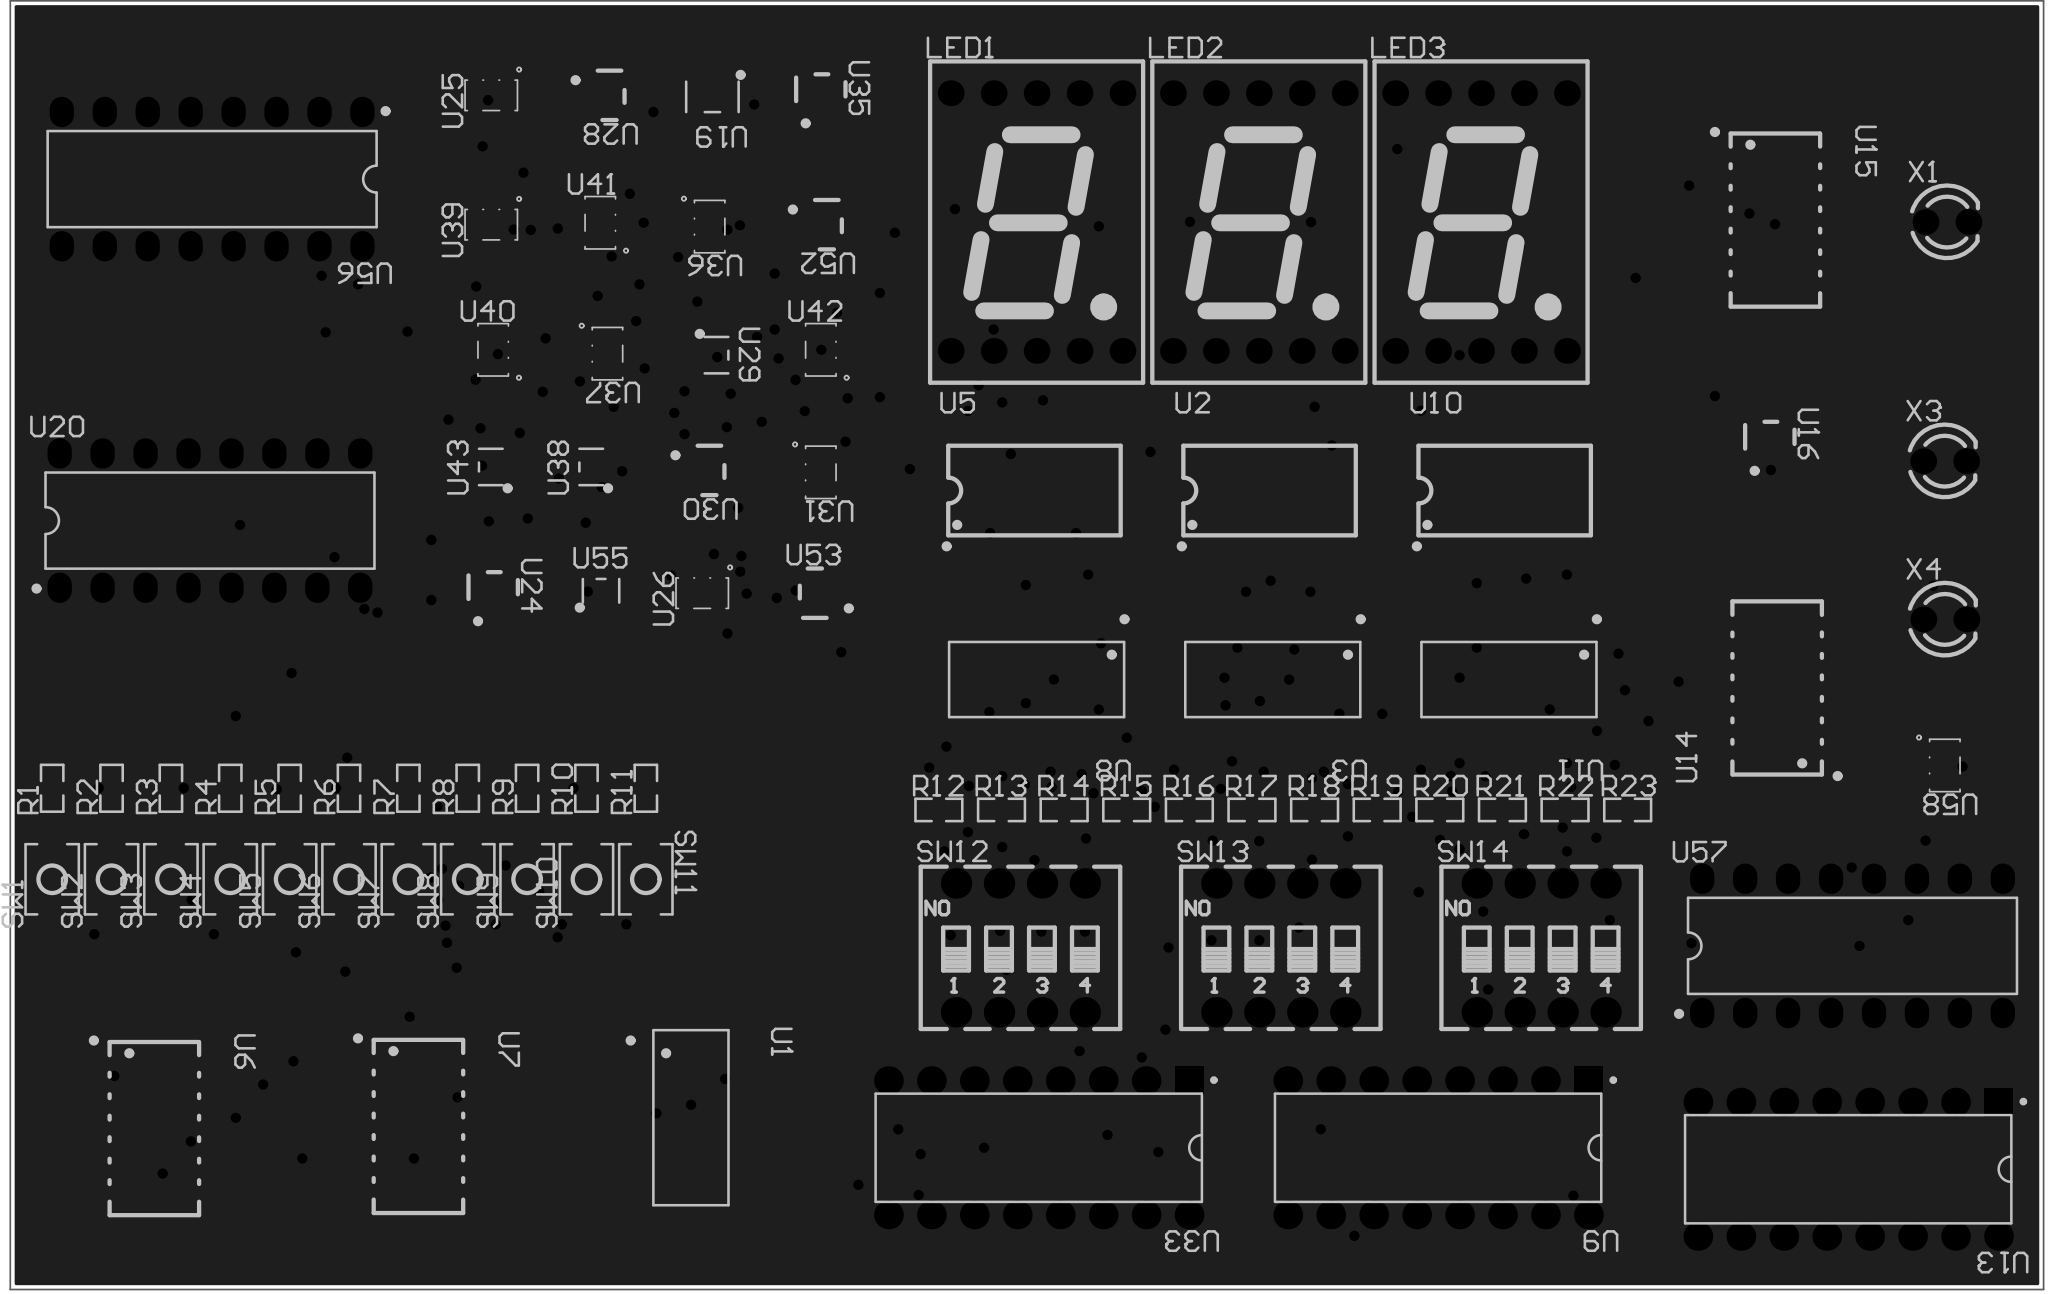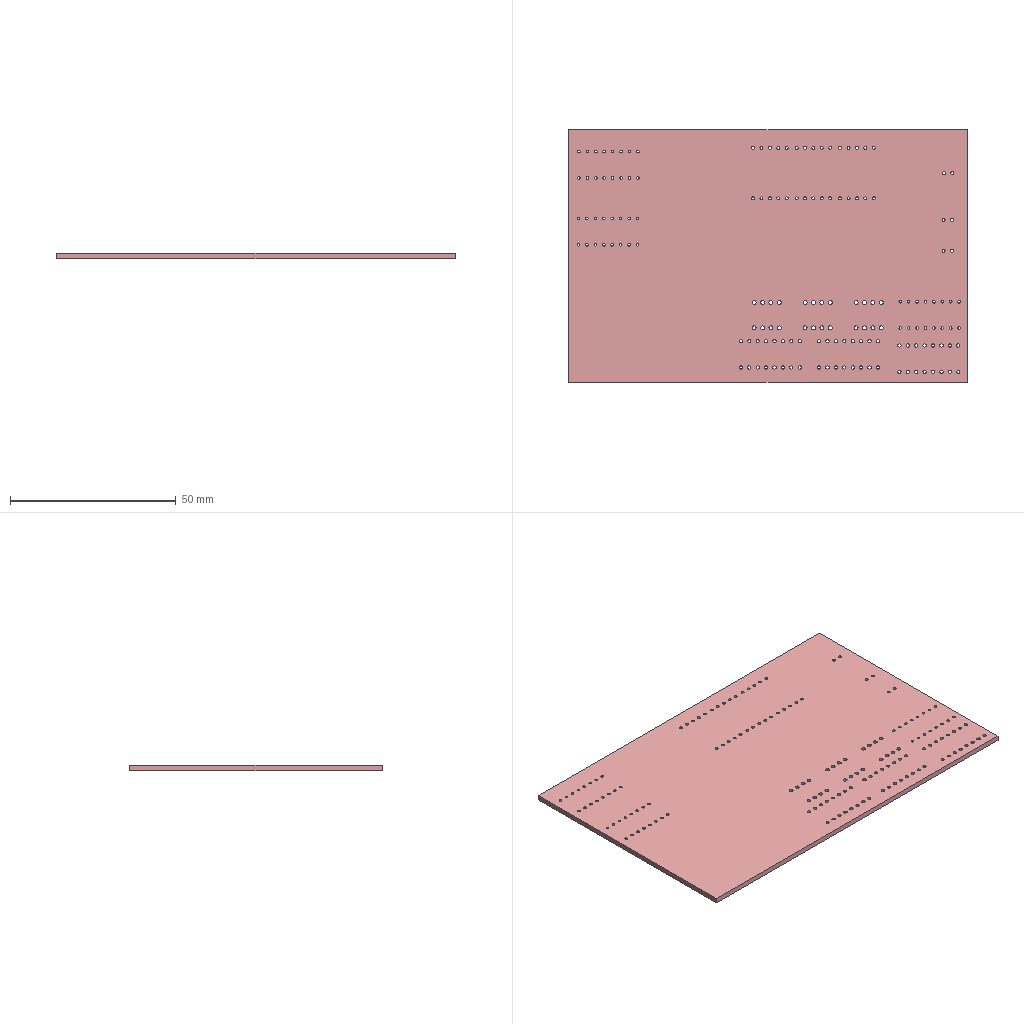Circuit board layout | Altium Designer | box 120.3 x 76.2 x 1.6 mm
Layer stack:
# Altium Designer layer stack of  (unit mm; dielectric type: 0 none, 1 core, 2 prepreg, 3 surface material)
index,name,kind,layer,copper_thickness_mm,dielectric_type,dielectric_thickness_mm,dielectric_material,dielectric_constant
0,Top Paste Mask Layer,other,,,,,,
1,Top Silkscreen Layer,other,,,,,,
2,Top Solder Mask Layer,dielectric,,,3,0.01,,3.3
3,Top Layer,copper,Top Layer,0.035,,,,
4,Dielectric1,dielectric,,,3,1.51,FR4,4.5
5,Bottom Layer,copper,Bottom Layer,0.035,,,,
6,Bottom Solder Mask Layer,dielectric,,,3,0.01,,3.3
7,Bottom Silkscreen Layer,other,,,,,,
8,Bottom Paste Mask Layer,other,,,,,,
# drill layer pairs: low layer,high layer
drill_pair,Top Layer,Bottom Layer
Part placement:
Designator,Comment,Layer,Footprint,Center-X(mm),Center-Y(mm),Rotation
LED1,,TopLayer,LED-SEG-TH_10P-L12.6-W19.0-P2.54-S15.24-BL,140.716,142.24,0
LED2,,TopLayer,LED-SEG-TH_10P-L12.6-W19.0-P2.54-S15.24-BL,153.861,142.24,0
LED3,,TopLayer,LED-SEG-TH_10P-L12.6-W19.0-P2.54-S15.24-BL,167.005,142.24,0
R1,1K,TopLayer,R0603,82.487,108.76,90
R2,1K,TopLayer,R0603,85.999,108.76,90
R3,1K,TopLayer,R0603,89.51,108.76,90
R4,1K,TopLayer,R0603,93.022,108.76,90
R5,1K,TopLayer,R0603,96.533,108.76,90
R6,1K,TopLayer,R0603,100.045,108.76,90
R7,1K,TopLayer,R0603,103.556,108.76,90
R8,1K,TopLayer,R0603,107.068,108.76,90
R9,1K,TopLayer,R0603,110.579,108.76,90
R10,1K,TopLayer,R0603,114.091,108.76,90
R11,1K,TopLayer,R0603,117.602,108.76,90
R12,1K,TopLayer,R0603,134.936,107.478,0
R13,1K,TopLayer,R0603,138.639,107.478,0
R14,1K,TopLayer,R0603,142.343,107.478,0
R15,1K,TopLayer,R0603,146.047,107.478,0
R16,1K,TopLayer,R0603,149.751,107.478,0
R17,1K,TopLayer,R0603,153.455,107.478,0
R18,1K,TopLayer,R0603,157.158,107.478,0
R19,1K,TopLayer,R0603,160.862,107.478,0
R20,1K,TopLayer,R0603,164.566,107.478,0
R21,1K,TopLayer,R0603,168.27,107.478,0
R22,1K,TopLayer,R0603,171.974,107.478,0
R23,1K,TopLayer,R0603,175.677,107.478,0
SW1,轻触按键3*4*H,TopLayer,SW-SMD_L4.0-W2.9-LS5.0,82.487,103.378,90
SW2,轻触按键3*4*H,TopLayer,SW-SMD_L4.0-W2.9-LS5.0,85.999,103.378,90
SW3,轻触按键3*4*H,TopLayer,SW-SMD_L4.0-W2.9-LS5.0,89.51,103.378,90
SW4,轻触按键3*4*H,TopLayer,SW-SMD_L4.0-W2.9-LS5.0,93.022,103.378,90
SW5,轻触按键3*4*H,TopLayer,SW-SMD_L4.0-W2.9-LS5.0,96.533,103.378,90
SW6,轻触按键3*4*H,TopLayer,SW-SMD_L4.0-W2.9-LS5.0,100.045,103.378,90
SW7,轻触按键3*4*H,TopLayer,SW-SMD_L4.0-W2.9-LS5.0,103.556,103.378,90
SW8,轻触按键3*4*H,TopLayer,SW-SMD_L4.0-W2.9-LS5.0,107.068,103.378,90
SW9,轻触按键3*4*H,TopLayer,SW-SMD_L4.0-W2.9-LS5.0,110.579,103.378,90
SW10,轻触按键3*4*H,TopLayer,SW-SMD_L4.0-W2.9-LS5.0,114.091,103.378,90
SW11,轻触按键3*4*H,TopLayer,SW-SMD_L4.0-W2.9-LS5.0,117.602,103.378,270
SW12,DSWB04LHGET,TopLayer,SW-TH_DSWB04LHGET,139.762,99.324,0
SW13,DSWB04LHGET,TopLayer,SW-TH_DSWB04LHGET,155.161,99.324,0
SW14,DSWB04LHGET,TopLayer,SW-TH_DSWB04LHGET,170.561,99.324,0
U1,SN74LS04NSR,TopLayer,SOIC-14_L10.0-W5.5-P1.27-LS7.8-BL,120.269,89.281,270
U2,SN74LS47NSR,TopLayer,SO-16_L10.2-W5.3-P1.27-LS7.8-BL,154.495,126.365,0
U3,SN74LS85NS,TopLayer,SOIC-16_L10.8-W5.5-P1.27-LS7.8-BL,154.686,115.189,180
U5,SN74LS47NSR,TopLayer,SO-16_L10.2-W5.3-P1.27-LS7.8-BL,140.589,126.365,0
U6,SN74HC21NSR,TopLayer,SO-14_L10.2-W5.3-P1.27-LS7.8-BL-1,88.519,88.646,270
U7,SN74HC21NSR,TopLayer,SO-14_L10.2-W5.3-P1.27-LS7.8-BL-1,104.14,88.773,270
U8,SN74LS85NS,TopLayer,SOIC-16_L10.8-W5.5-P1.27-LS7.8-BL,140.716,115.189,180
U9,SN74S175N,TopLayer,PDIP-16_L19.3-W6.4-P2.54-LS7.9-BL,164.465,87.503,180
U10,SN74LS47NSR,TopLayer,SO-16_L10.2-W5.3-P1.27-LS7.8-BL,168.402,126.365,0
U11,SN74LS85NS,TopLayer,SOIC-16_L10.8-W5.5-P1.27-LS7.8-BL,168.656,115.189,180
U13,SN74S175N,TopLayer,PDIP-16_L19.3-W6.4-P2.54-LS7.9-BL,188.722,86.233,180
U14,SN74HC21NSR,TopLayer,SO-14_L10.2-W5.3-P1.27-LS7.8-BL-1,184.531,114.681,90
U15,SN74HC21NSR,TopLayer,SO-14_L10.2-W5.3-P1.27-LS7.8-BL-1,184.404,142.367,270
U16,NC7SU04M5-FS,TopLayer,SOT-23-5_L2.9-W1.6-P0.95-LS2.8-BR,184.15,129.54,270
U19,NC7S08M5,TopLayer,SOT-23-5_L3.0-W1.5-P0.95-LS2.8-BL,121.539,149.643,180
U20,SN74LS147N(LX),TopLayer,PDIP-16_L19.3-W6.4-P2.54-LS7.94-BL,91.821,124.587,0
U24,NC7SU04M5-FS,TopLayer,SOT-23-5_L2.9-W1.6-P0.95-LS2.8-BR,108.636,120.65,270
U25,NC7S08M5X,TopLayer,SOT-23-5_L3.0-W1.7-P0.95-LS2.8-BR,108.458,149.733,90
U26,NC7S08M5X,TopLayer,SOT-23-5_L3.0-W1.7-P0.95-LS2.8-BR,120.937,120.295,90
U28,NC7SU04M5-FS,TopLayer,SOT-23-5_L2.9-W1.6-P0.95-LS2.8-BR,115.454,149.669,180
U29,NC7S02P5X,TopLayer,SC-70-5_L2.1-W1.3-P0.65-LS2.1-BL,121.783,134.369,270
U30,NC7SU04M5-FS,TopLayer,SOT-23-5_L2.9-W1.6-P0.95-LS2.8-BR,121.363,127.491,180
U31,NC7S08M5X,TopLayer,SOT-23-5_L3.0-W1.7-P0.95-LS2.8-BR,127.953,127.44,180
U33,SN74S175N,TopLayer,PDIP-16_L19.3-W6.4-P2.54-LS7.9-BL,140.843,87.503,180
U35,NC7SU04M5-FS,TopLayer,SOT-23-5_L2.9-W1.6-P0.95-LS2.8-BR,128.016,150.088,270
U36,NC7S08M5X,TopLayer,SOT-23-5_L3.0-W1.7-P0.95-LS2.8-BR,121.377,141.971,180
U37,NC7S08M5X,TopLayer,SOT-23-5_L3.0-W1.7-P0.95-LS2.8-BR,115.332,134.458,180
U38,NC7S02P5X,TopLayer,SC-70-5_L2.1-W1.3-P0.65-LS2.1-BL,114.372,127.758,90
U39,NC7S08M5X,TopLayer,SOT-23-5_L3.0-W1.7-P0.95-LS2.8-BR,108.458,142.085,90
U40,NC7S08M5X,TopLayer,SOT-23-5_L3.0-W1.7-P0.95-LS2.8-BR,108.572,134.687,0
U41,NC7S08M5X,TopLayer,SOT-23-5_L3.0-W1.7-P0.95-LS2.8-BR,114.906,142.199,0
U42,NC7S08M5X,TopLayer,SOT-23-5_L3.0-W1.7-P0.95-LS2.8-BR,127.953,134.687,0
U43,NC7S02P5X,TopLayer,SC-70-5_L2.1-W1.3-P0.65-LS2.1-BL,108.432,127.758,90
U52,NC7SU04M5-FS,TopLayer,SOT-23-5_L2.9-W1.6-P0.95-LS2.8-BR,128.308,142.021,180
U53,NC7SU04M5-FS,TopLayer,SOT-23-5_L2.9-W1.6-P0.95-LS2.8-BR,127.597,120.359,0
U55,NC7S02P5X,TopLayer,SC-70-5_L2.1-W1.3-P0.65-LS2.1-BL,114.952,120.435,0
U56,SN74LS161N(LX),TopLayer,PDIP-16_L19.3-W6.4-P2.54-LS7.94-BL,91.948,144.78,180
U57,SN74LS161N(LX),TopLayer,PDIP-16_L19.3-W6.4-P2.54-LS7.94-BL,188.976,99.441,0
U58,NC7S08M5X,TopLayer,SOT-23-5_L3.0-W1.7-P0.95-LS2.8-BR,194.437,110.109,180
X4,,TopLayer,LED_TH-3mm,194.437,118.745,0
X1,,TopLayer,LED_TH-3mm,194.564,142.24,0
X3,,TopLayer,LED_TH-3mm,194.429,128.103,0
Pad and via stacks:
# Altium Designer via and pad stacks of  (unit mm). Each distinct definition once, with the count of objects using it.
# via: kind,start_layer,end_layer,hole_mm,diameter_mm,mode(0 simple;1 top-mid-bottom;2 full stack),diameter_per_layer,count,example_net
# pad: kind,layer,hole_mm,hole_type(0 round;1 square;2 slot),plating,top_size,top_shape(1 round;2 rect;3 octagon;9 rounded rect),mid_size,bottom_size,mode,footprint,size_per_layer,count,example
pad,Multi-Layer,0.9144,0,plated,1.524x1.524,1,1.524x1.524,1.524x1.524,0,LED-SEG-TH_10P-L12.6-W19.0-P2.54-S15.24-BL,,30,LED1.1
pad,Multi-Layer,1.2,0,plated,1.8x1.8,1,1.8x1.8,1.8x1.8,0,SW-TH_DSWB04LHGET,,24,SW12.5
pad,Multi-Layer,1,0,plated,1.7x1.7,2,1.7x1.7,1.7x1.7,0,PDIP-16_L19.3-W6.4-P2.54-LS7.9-BL,,3,U9.1
pad,Multi-Layer,1,0,plated,1.7x1.7,1,1.7x1.7,1.7x1.7,0,PDIP-16_L19.3-W6.4-P2.54-LS7.9-BL,,45,U9.2
pad,Multi-Layer,0.8,0,plated,1.44x1.8,1,1.44x1.8,1.44x1.8,0,PDIP-16_L19.3-W6.4-P2.54-LS7.94-BL,,48,U20.1
pad,Multi-Layer,0.9144,0,plated,1.524x1.524,1,1.524x1.524,1.524x1.524,0,LED_TH-3mm,,6,X4.1
pad,Top Layer,0,0,plated,0.8065x0.864,2,0.8065x0.864,0.8065x0.864,0,R0603,,46,R1.2
pad,Top Layer,0,0,plated,1.53x1.36,2,1.53x1.36,1.53x1.36,0,SW-SMD_L4.0-W2.9-LS5.0,,22,SW1.1
pad,Top Layer,0,0,plated,0.602x2.231,1,0.602x2.231,0.602x2.231,0,SOIC-14_L10.0-W5.5-P1.27-LS7.8-BL,,14,U1.1
pad,Top Layer,0,0,plated,0.595x1.597,1,0.595x1.597,0.595x1.597,0,SO-16_L10.2-W5.3-P1.27-LS7.8-BL,,48,U2.9
pad,Top Layer,0,0,plated,0.602x2.231,1,0.602x2.231,0.602x2.231,0,SOIC-16_L10.8-W5.5-P1.27-LS7.8-BL,,48,U3.1
pad,Top Layer,0,0,plated,0.602x2.231,1,0.602x2.231,0.602x2.231,0,SO-14_L10.2-W5.3-P1.27-LS7.8-BL-1,,56,U6.1
pad,Top Layer,0,0,plated,0.6x1,2,0.6x1,0.6x1,0,SOT-23-5_L2.9-W1.6-P0.95-LS2.8-BR,,35,U16.2
pad,Top Layer,0,0,plated,0.532x1.045,2,0.532x1.045,0.532x1.045,0,SOT-23-5_L3.0-W1.5-P0.95-LS2.8-BL,,5,U19.5
pad,Top Layer,0,0,plated,1.1x0.6,2,1.1x0.6,1.1x0.6,0,SOT-23-5_L3.0-W1.7-P0.95-LS2.8-BR,,50,U25.5
pad,Top Layer,0,0,plated,0.315x0.835,2,0.315x0.835,0.315x0.835,0,SC-70-5_L2.1-W1.3-P0.65-LS2.1-BL,,20,U29.1
via,Top Layer,Bottom Layer,0.3048,0.61,0,,251,$1N10282
Copper pours:
name,layer,net,type(0 solid;1 hatched;2 none)
Top Layer-GND,Top Layer,GND,0
Bottom Layer-GND,Bottom Layer,GND,0